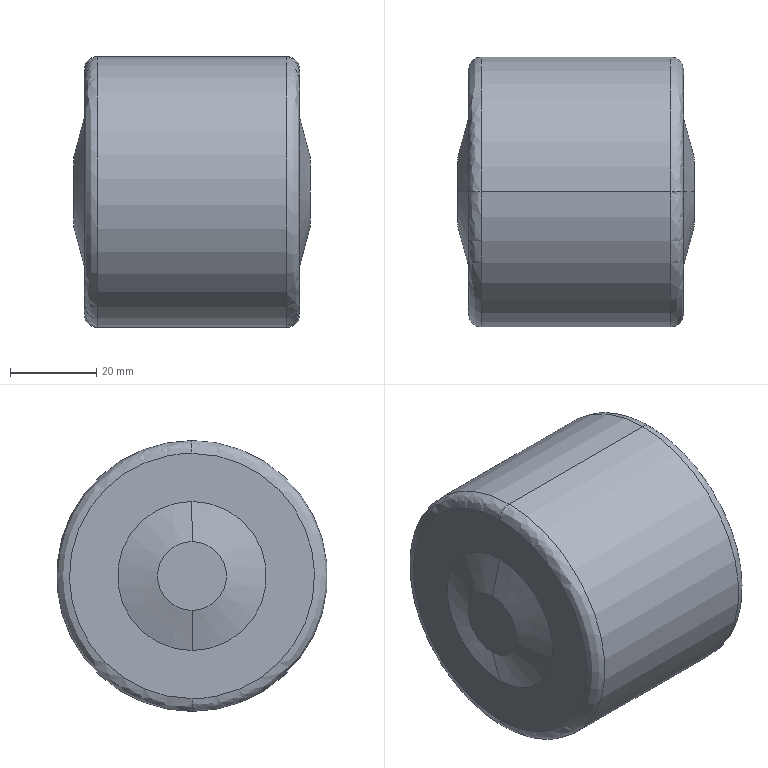Part | SolidWorks | features BaseBody 1 | 1 solid | 14 faces | box 55 x 63 x 63 mm | volume 157755 mm3 | spline 4 | cone 4 | plane 4 | cylinder 2 | commonest cylinder face diameters 63 x2
STEP:
#1=CARTESIAN_POINT('',(-22.,0.,31.5));
#2=VERTEX_POINT('',#1);
#3=CARTESIAN_POINT('',(-22.,0.,-31.5));
#4=VERTEX_POINT('',#3);
#5=CARTESIAN_POINT('',(-22.,0.,0.));
#6=DIRECTION('',(1.,0.,0.));
#7=DIRECTION('',(0.,0.,1.));
#8=AXIS2_PLACEMENT_3D('',#5,#6,#7);
#9=CIRCLE('',#8,31.5);
#10=EDGE_CURVE('',#2,#4,#9,.T.);
#11=ORIENTED_EDGE('',*,*,#10,.F.);
#12=CARTESIAN_POINT('',(-25.,0.,28.5));
#13=VERTEX_POINT('',#12);
#14=CARTESIAN_POINT('',(-22.,0.,28.5));
#15=DIRECTION('',(0.,-1.,0.));
#16=DIRECTION('',(0.,0.,1.));
#17=AXIS2_PLACEMENT_3D('',#14,#15,#16);
#18=CIRCLE('',#17,3.);
#19=EDGE_CURVE('',#2,#13,#18,.T.);
#20=ORIENTED_EDGE('',*,*,#19,.T.);
#21=CARTESIAN_POINT('',(-25.,0.,-28.5));
#22=VERTEX_POINT('',#21);
#23=CARTESIAN_POINT('',(-25.,0.,28.5));
#24=CARTESIAN_POINT('',(-25.,-57.,28.5));
#25=CARTESIAN_POINT('',(-25.,-57.,-28.5));
#26=CARTESIAN_POINT('',(-25.,0.,-28.5));
#27=(BOUNDED_CURVE()B_SPLINE_CURVE(3,(#23,#24,#25,#26),.UNSPECIFIED.,.F.,.T.)B_SPLINE_CURVE_WITH_KNOTS((4,4),(0.5,1.),.UNSPECIFIED.)CURVE()GEOMETRIC_REPRESENTATION_ITEM()RATIONAL_B_SPLINE_CURVE((1.,0.3333,0.3333,1.))REPRESENTATION_ITEM(''));
#28=EDGE_CURVE('',#13,#22,#27,.T.);
#29=ORIENTED_EDGE('',*,*,#28,.T.);
#30=CARTESIAN_POINT('',(-22.,0.,-28.5));
#31=DIRECTION('',(0.,1.,0.));
#32=DIRECTION('',(0.,0.,-1.));
#33=AXIS2_PLACEMENT_3D('',#30,#31,#32);
#34=CIRCLE('',#33,3.);
#35=EDGE_CURVE('',#4,#22,#34,.T.);
#36=ORIENTED_EDGE('',*,*,#35,.F.);
#37=EDGE_LOOP('',(#11,#20,#29,#36));
#38=FACE_OUTER_BOUND('',#37,.T.);
#39=CARTESIAN_POINT('',(-22.,0.,31.5));
#40=CARTESIAN_POINT('',(-22.,-63.,31.5));
#41=CARTESIAN_POINT('',(-22.,-63.,-31.5));
#42=CARTESIAN_POINT('',(-22.,0.,-31.5));
#43=CARTESIAN_POINT('',(-23.757,0.,31.5));
#44=CARTESIAN_POINT('',(-23.757,-63.,31.5));
#45=CARTESIAN_POINT('',(-23.757,-63.,-31.5));
#46=CARTESIAN_POINT('',(-23.757,0.,-31.5));
#47=CARTESIAN_POINT('',(-25.,0.,30.257));
#48=CARTESIAN_POINT('',(-25.,-60.515,30.257));
#49=CARTESIAN_POINT('',(-25.,-60.515,-30.257));
#50=CARTESIAN_POINT('',(-25.,0.,-30.257));
#51=CARTESIAN_POINT('',(-25.,0.,28.5));
#52=CARTESIAN_POINT('',(-25.,-57.,28.5));
#53=CARTESIAN_POINT('',(-25.,-57.,-28.5));
#54=CARTESIAN_POINT('',(-25.,0.,-28.5));
#55=(BOUNDED_SURFACE()B_SPLINE_SURFACE(3,3,((#39,#40,#41,#42),(#43,#44,#45,#46),(#47,#48,#49,#50),(#51,#52,#53,#54)),.UNSPECIFIED.,.F.,.F.,.F.)B_SPLINE_SURFACE_WITH_KNOTS((4,4),(4,4),(0.,1.),(0.,1.),.UNSPECIFIED.)GEOMETRIC_REPRESENTATION_ITEM()RATIONAL_B_SPLINE_SURFACE(((1.,0.3333,0.3333,1.),(0.8047,0.2682,0.2682,0.8047),(0.8047,0.2682,0.2682,0.8047),(1.,0.3333,0.3333,1.)))REPRESENTATION_ITEM('')SURFACE());
#56=ADVANCED_FACE('',(#38),#55,.T.);
#57=CARTESIAN_POINT('',(25.,0.,-28.5));
#58=VERTEX_POINT('',#57);
#59=CARTESIAN_POINT('',(25.,0.,28.5));
#60=VERTEX_POINT('',#59);
#61=CARTESIAN_POINT('',(25.,0.,-28.5));
#62=CARTESIAN_POINT('',(25.,-57.,-28.5));
#63=CARTESIAN_POINT('',(25.,-57.,28.5));
#64=CARTESIAN_POINT('',(25.,0.,28.5));
#65=(BOUNDED_CURVE()B_SPLINE_CURVE(3,(#61,#62,#63,#64),.UNSPECIFIED.,.F.,.F.)B_SPLINE_CURVE_WITH_KNOTS((4,4),(0.,0.5),.UNSPECIFIED.)CURVE()GEOMETRIC_REPRESENTATION_ITEM()RATIONAL_B_SPLINE_CURVE((1.,0.3333,0.3333,1.))REPRESENTATION_ITEM(''));
#66=EDGE_CURVE('',#58,#60,#65,.T.);
#67=ORIENTED_EDGE('',*,*,#66,.T.);
#68=CARTESIAN_POINT('',(22.,0.,31.5));
#69=VERTEX_POINT('',#68);
#70=CARTESIAN_POINT('',(22.,0.,28.5));
#71=DIRECTION('',(0.,-1.,0.));
#72=DIRECTION('',(0.,0.,1.));
#73=AXIS2_PLACEMENT_3D('',#70,#71,#72);
#74=CIRCLE('',#73,3.);
#75=EDGE_CURVE('',#60,#69,#74,.T.);
#76=ORIENTED_EDGE('',*,*,#75,.T.);
#77=CARTESIAN_POINT('',(22.,0.,-31.5));
#78=VERTEX_POINT('',#77);
#79=CARTESIAN_POINT('',(22.,0.,0.));
#80=DIRECTION('',(-1.,0.,0.));
#81=DIRECTION('',(0.,0.,1.));
#82=AXIS2_PLACEMENT_3D('',#79,#80,#81);
#83=CIRCLE('',#82,31.5);
#84=EDGE_CURVE('',#78,#69,#83,.T.);
#85=ORIENTED_EDGE('',*,*,#84,.F.);
#86=CARTESIAN_POINT('',(22.,0.,-28.5));
#87=DIRECTION('',(0.,1.,0.));
#88=DIRECTION('',(0.,0.,-1.));
#89=AXIS2_PLACEMENT_3D('',#86,#87,#88);
#90=CIRCLE('',#89,3.);
#91=EDGE_CURVE('',#58,#78,#90,.T.);
#92=ORIENTED_EDGE('',*,*,#91,.F.);
#93=EDGE_LOOP('',(#67,#76,#85,#92));
#94=FACE_OUTER_BOUND('',#93,.T.);
#95=CARTESIAN_POINT('',(25.,0.,28.5));
#96=CARTESIAN_POINT('',(25.,-57.,28.5));
#97=CARTESIAN_POINT('',(25.,-57.,-28.5));
#98=CARTESIAN_POINT('',(25.,0.,-28.5));
#99=CARTESIAN_POINT('',(25.,0.,30.257));
#100=CARTESIAN_POINT('',(25.,-60.515,30.257));
#101=CARTESIAN_POINT('',(25.,-60.515,-30.257));
#102=CARTESIAN_POINT('',(25.,0.,-30.257));
#103=CARTESIAN_POINT('',(23.757,0.,31.5));
#104=CARTESIAN_POINT('',(23.757,-63.,31.5));
#105=CARTESIAN_POINT('',(23.757,-63.,-31.5));
#106=CARTESIAN_POINT('',(23.757,0.,-31.5));
#107=CARTESIAN_POINT('',(22.,0.,31.5));
#108=CARTESIAN_POINT('',(22.,-63.,31.5));
#109=CARTESIAN_POINT('',(22.,-63.,-31.5));
#110=CARTESIAN_POINT('',(22.,0.,-31.5));
#111=(BOUNDED_SURFACE()B_SPLINE_SURFACE(3,3,((#95,#96,#97,#98),(#99,#100,#101,#102),(#103,#104,#105,#106),(#107,#108,#109,#110)),.UNSPECIFIED.,.F.,.F.,.T.)B_SPLINE_SURFACE_WITH_KNOTS((4,4),(4,4),(0.,1.),(0.,1.),.UNSPECIFIED.)GEOMETRIC_REPRESENTATION_ITEM()RATIONAL_B_SPLINE_SURFACE(((1.,0.3333,0.3333,1.),(0.8047,0.2682,0.2682,0.8047),(0.8047,0.2682,0.2682,0.8047),(1.,0.3333,0.3333,1.)))REPRESENTATION_ITEM('')SURFACE());
#112=ADVANCED_FACE('',(#94),#111,.T.);
#113=CARTESIAN_POINT('',(22.,0.,0.));
#114=DIRECTION('',(-1.,0.,0.));
#115=DIRECTION('',(0.,0.,1.));
#116=AXIS2_PLACEMENT_3D('',#113,#114,#115);
#117=CIRCLE('',#116,31.5);
#118=EDGE_CURVE('',#69,#78,#117,.T.);
#119=ORIENTED_EDGE('',*,*,#118,.T.);
#120=CARTESIAN_POINT('',(50.,0.,-31.5));
#121=DIRECTION('',(-1.,0.,0.));
#122=VECTOR('',#121,1000.);
#123=LINE('',#120,#122);
#124=EDGE_CURVE('',#78,#4,#123,.T.);
#125=ORIENTED_EDGE('',*,*,#124,.T.);
#126=CARTESIAN_POINT('',(-22.,0.,0.));
#127=DIRECTION('',(1.,0.,0.));
#128=DIRECTION('',(0.,0.,1.));
#129=AXIS2_PLACEMENT_3D('',#126,#127,#128);
#130=CIRCLE('',#129,31.5);
#131=EDGE_CURVE('',#4,#2,#130,.T.);
#132=ORIENTED_EDGE('',*,*,#131,.T.);
#133=CARTESIAN_POINT('',(50.,0.,31.5));
#134=DIRECTION('',(-1.,0.,0.));
#135=VECTOR('',#134,1000.);
#136=LINE('',#133,#135);
#137=EDGE_CURVE('',#69,#2,#136,.T.);
#138=ORIENTED_EDGE('',*,*,#137,.F.);
#139=EDGE_LOOP('',(#119,#125,#132,#138));
#140=FACE_OUTER_BOUND('',#139,.T.);
#141=CARTESIAN_POINT('',(50.,0.,0.));
#142=DIRECTION('',(-1.,0.,0.));
#143=DIRECTION('',(0.,0.,1.));
#144=AXIS2_PLACEMENT_3D('',#141,#142,#143);
#145=CYLINDRICAL_SURFACE('',#144,31.5);
#146=ADVANCED_FACE('',(#140),#145,.T.);
#147=CARTESIAN_POINT('',(-27.5,0.,-8.));
#148=VERTEX_POINT('',#147);
#149=CARTESIAN_POINT('',(-27.5,0.,8.));
#150=VERTEX_POINT('',#149);
#151=CARTESIAN_POINT('',(-27.5,0.,0.));
#152=DIRECTION('',(1.,0.,0.));
#153=DIRECTION('',(0.,0.,-1.));
#154=AXIS2_PLACEMENT_3D('',#151,#152,#153);
#155=CIRCLE('',#154,8.);
#156=EDGE_CURVE('',#148,#150,#155,.T.);
#157=ORIENTED_EDGE('',*,*,#156,.T.);
#158=CARTESIAN_POINT('',(-25.,0.,17.33));
#159=VERTEX_POINT('',#158);
#160=CARTESIAN_POINT('',(-25.,0.,17.33));
#161=DIRECTION('',(0.2588,0.,0.9659));
#162=VECTOR('',#161,1000.);
#163=LINE('',#160,#162);
#164=EDGE_CURVE('',#150,#159,#163,.T.);
#165=ORIENTED_EDGE('',*,*,#164,.T.);
#166=CARTESIAN_POINT('',(-25.,0.,-17.33));
#167=VERTEX_POINT('',#166);
#168=CARTESIAN_POINT('',(-25.,0.,0.));
#169=DIRECTION('',(-1.,0.,0.));
#170=DIRECTION('',(0.,0.,-1.));
#171=AXIS2_PLACEMENT_3D('',#168,#169,#170);
#172=CIRCLE('',#171,17.33);
#173=EDGE_CURVE('',#159,#167,#172,.T.);
#174=ORIENTED_EDGE('',*,*,#173,.T.);
#175=CARTESIAN_POINT('',(-25.,0.,-17.33));
#176=DIRECTION('',(0.2588,0.,-0.9659));
#177=VECTOR('',#176,1000.);
#178=LINE('',#175,#177);
#179=EDGE_CURVE('',#148,#167,#178,.T.);
#180=ORIENTED_EDGE('',*,*,#179,.F.);
#181=EDGE_LOOP('',(#157,#165,#174,#180));
#182=FACE_OUTER_BOUND('',#181,.T.);
#183=CARTESIAN_POINT('',(-25.,0.,0.));
#184=DIRECTION('',(1.,0.,0.));
#185=DIRECTION('',(0.,0.,-1.));
#186=AXIS2_PLACEMENT_3D('',#183,#184,#185);
#187=CONICAL_SURFACE('',#186,17.33,1.309);
#188=ADVANCED_FACE('',(#182),#187,.T.);
#189=CARTESIAN_POINT('',(27.5,0.,8.));
#190=VERTEX_POINT('',#189);
#191=CARTESIAN_POINT('',(27.5,0.,-8.));
#192=VERTEX_POINT('',#191);
#193=CARTESIAN_POINT('',(27.5,0.,0.));
#194=DIRECTION('',(-1.,0.,0.));
#195=DIRECTION('',(0.,0.,1.));
#196=AXIS2_PLACEMENT_3D('',#193,#194,#195);
#197=CIRCLE('',#196,8.);
#198=EDGE_CURVE('',#190,#192,#197,.T.);
#199=ORIENTED_EDGE('',*,*,#198,.T.);
#200=CARTESIAN_POINT('',(25.,0.,-17.33));
#201=VERTEX_POINT('',#200);
#202=CARTESIAN_POINT('',(25.,0.,-17.33));
#203=DIRECTION('',(-0.2588,0.,-0.9659));
#204=VECTOR('',#203,1000.);
#205=LINE('',#202,#204);
#206=EDGE_CURVE('',#192,#201,#205,.T.);
#207=ORIENTED_EDGE('',*,*,#206,.T.);
#208=CARTESIAN_POINT('',(25.,0.,17.33));
#209=VERTEX_POINT('',#208);
#210=CARTESIAN_POINT('',(25.,0.,0.));
#211=DIRECTION('',(1.,0.,0.));
#212=DIRECTION('',(0.,0.,1.));
#213=AXIS2_PLACEMENT_3D('',#210,#211,#212);
#214=CIRCLE('',#213,17.33);
#215=EDGE_CURVE('',#201,#209,#214,.T.);
#216=ORIENTED_EDGE('',*,*,#215,.T.);
#217=CARTESIAN_POINT('',(25.,0.,17.33));
#218=DIRECTION('',(-0.2588,0.,0.9659));
#219=VECTOR('',#218,1000.);
#220=LINE('',#217,#219);
#221=EDGE_CURVE('',#190,#209,#220,.T.);
#222=ORIENTED_EDGE('',*,*,#221,.F.);
#223=EDGE_LOOP('',(#199,#207,#216,#222));
#224=FACE_OUTER_BOUND('',#223,.T.);
#225=CARTESIAN_POINT('',(25.,0.,0.));
#226=DIRECTION('',(-1.,0.,0.));
#227=DIRECTION('',(0.,0.,1.));
#228=AXIS2_PLACEMENT_3D('',#225,#226,#227);
#229=CONICAL_SURFACE('',#228,17.33,1.309);
#230=ADVANCED_FACE('',(#224),#229,.T.);
#231=ORIENTED_EDGE('',*,*,#124,.F.);
#232=ORIENTED_EDGE('',*,*,#84,.T.);
#233=ORIENTED_EDGE('',*,*,#137,.T.);
#234=ORIENTED_EDGE('',*,*,#10,.T.);
#235=EDGE_LOOP('',(#231,#232,#233,#234));
#236=FACE_OUTER_BOUND('',#235,.T.);
#237=CARTESIAN_POINT('',(50.,0.,0.));
#238=DIRECTION('',(-1.,0.,0.));
#239=DIRECTION('',(0.,0.,1.));
#240=AXIS2_PLACEMENT_3D('',#237,#238,#239);
#241=CYLINDRICAL_SURFACE('',#240,31.5);
#242=ADVANCED_FACE('',(#236),#241,.T.);
#243=ORIENTED_EDGE('',*,*,#19,.F.);
#244=ORIENTED_EDGE('',*,*,#131,.F.);
#245=ORIENTED_EDGE('',*,*,#35,.T.);
#246=CARTESIAN_POINT('',(-25.,0.,-28.5));
#247=CARTESIAN_POINT('',(-25.,57.,-28.5));
#248=CARTESIAN_POINT('',(-25.,57.,28.5));
#249=CARTESIAN_POINT('',(-25.,0.,28.5));
#250=(BOUNDED_CURVE()B_SPLINE_CURVE(3,(#246,#247,#248,#249),.UNSPECIFIED.,.F.,.T.)B_SPLINE_CURVE_WITH_KNOTS((4,4),(0.,0.5),.UNSPECIFIED.)CURVE()GEOMETRIC_REPRESENTATION_ITEM()RATIONAL_B_SPLINE_CURVE((1.,0.3333,0.3333,1.))REPRESENTATION_ITEM(''));
#251=EDGE_CURVE('',#22,#13,#250,.T.);
#252=ORIENTED_EDGE('',*,*,#251,.T.);
#253=EDGE_LOOP('',(#243,#244,#245,#252));
#254=FACE_OUTER_BOUND('',#253,.T.);
#255=CARTESIAN_POINT('',(-22.,0.,-31.5));
#256=CARTESIAN_POINT('',(-22.,63.,-31.5));
#257=CARTESIAN_POINT('',(-22.,63.,31.5));
#258=CARTESIAN_POINT('',(-22.,0.,31.5));
#259=CARTESIAN_POINT('',(-23.757,0.,-31.5));
#260=CARTESIAN_POINT('',(-23.757,63.,-31.5));
#261=CARTESIAN_POINT('',(-23.757,63.,31.5));
#262=CARTESIAN_POINT('',(-23.757,0.,31.5));
#263=CARTESIAN_POINT('',(-25.,0.,-30.257));
#264=CARTESIAN_POINT('',(-25.,60.515,-30.257));
#265=CARTESIAN_POINT('',(-25.,60.515,30.257));
#266=CARTESIAN_POINT('',(-25.,0.,30.257));
#267=CARTESIAN_POINT('',(-25.,0.,-28.5));
#268=CARTESIAN_POINT('',(-25.,57.,-28.5));
#269=CARTESIAN_POINT('',(-25.,57.,28.5));
#270=CARTESIAN_POINT('',(-25.,0.,28.5));
#271=(BOUNDED_SURFACE()B_SPLINE_SURFACE(3,3,((#255,#256,#257,#258),(#259,#260,#261,#262),(#263,#264,#265,#266),(#267,#268,#269,#270)),.UNSPECIFIED.,.F.,.F.,.F.)B_SPLINE_SURFACE_WITH_KNOTS((4,4),(4,4),(0.,1.),(0.,1.),.UNSPECIFIED.)GEOMETRIC_REPRESENTATION_ITEM()RATIONAL_B_SPLINE_SURFACE(((1.,0.3333,0.3333,1.),(0.8047,0.2682,0.2682,0.8047),(0.8047,0.2682,0.2682,0.8047),(1.,0.3333,0.3333,1.)))REPRESENTATION_ITEM('')SURFACE());
#272=ADVANCED_FACE('',(#254),#271,.T.);
#273=ORIENTED_EDGE('',*,*,#75,.F.);
#274=CARTESIAN_POINT('',(25.,0.,28.5));
#275=CARTESIAN_POINT('',(25.,57.,28.5));
#276=CARTESIAN_POINT('',(25.,57.,-28.5));
#277=CARTESIAN_POINT('',(25.,0.,-28.5));
#278=(BOUNDED_CURVE()B_SPLINE_CURVE(3,(#274,#275,#276,#277),.UNSPECIFIED.,.F.,.T.)B_SPLINE_CURVE_WITH_KNOTS((4,4),(0.5,1.),.UNSPECIFIED.)CURVE()GEOMETRIC_REPRESENTATION_ITEM()RATIONAL_B_SPLINE_CURVE((1.,0.3333,0.3333,1.))REPRESENTATION_ITEM(''));
#279=EDGE_CURVE('',#60,#58,#278,.T.);
#280=ORIENTED_EDGE('',*,*,#279,.T.);
#281=ORIENTED_EDGE('',*,*,#91,.T.);
#282=ORIENTED_EDGE('',*,*,#118,.F.);
#283=EDGE_LOOP('',(#273,#280,#281,#282));
#284=FACE_OUTER_BOUND('',#283,.T.);
#285=CARTESIAN_POINT('',(25.,0.,-28.5));
#286=CARTESIAN_POINT('',(25.,57.,-28.5));
#287=CARTESIAN_POINT('',(25.,57.,28.5));
#288=CARTESIAN_POINT('',(25.,0.,28.5));
#289=CARTESIAN_POINT('',(25.,0.,-30.257));
#290=CARTESIAN_POINT('',(25.,60.515,-30.257));
#291=CARTESIAN_POINT('',(25.,60.515,30.257));
#292=CARTESIAN_POINT('',(25.,0.,30.257));
#293=CARTESIAN_POINT('',(23.757,0.,-31.5));
#294=CARTESIAN_POINT('',(23.757,63.,-31.5));
#295=CARTESIAN_POINT('',(23.757,63.,31.5));
#296=CARTESIAN_POINT('',(23.757,0.,31.5));
#297=CARTESIAN_POINT('',(22.,0.,-31.5));
#298=CARTESIAN_POINT('',(22.,63.,-31.5));
#299=CARTESIAN_POINT('',(22.,63.,31.5));
#300=CARTESIAN_POINT('',(22.,0.,31.5));
#301=(BOUNDED_SURFACE()B_SPLINE_SURFACE(3,3,((#285,#286,#287,#288),(#289,#290,#291,#292),(#293,#294,#295,#296),(#297,#298,#299,#300)),.UNSPECIFIED.,.F.,.F.,.T.)B_SPLINE_SURFACE_WITH_KNOTS((4,4),(4,4),(0.,1.),(0.,1.),.UNSPECIFIED.)GEOMETRIC_REPRESENTATION_ITEM()RATIONAL_B_SPLINE_SURFACE(((1.,0.3333,0.3333,1.),(0.8047,0.2682,0.2682,0.8047),(0.8047,0.2682,0.2682,0.8047),(1.,0.3333,0.3333,1.)))REPRESENTATION_ITEM('')SURFACE());
#302=ADVANCED_FACE('',(#284),#301,.T.);
#303=CARTESIAN_POINT('',(-25.,0.,0.));
#304=DIRECTION('',(-1.,0.,0.));
#305=DIRECTION('',(0.,0.,-1.));
#306=AXIS2_PLACEMENT_3D('',#303,#304,#305);
#307=CIRCLE('',#306,17.33);
#308=EDGE_CURVE('',#167,#159,#307,.T.);
#309=ORIENTED_EDGE('',*,*,#308,.F.);
#310=ORIENTED_EDGE('',*,*,#173,.F.);
#311=EDGE_LOOP('',(#309,#310));
#312=FACE_BOUND('',#311,.T.);
#313=ORIENTED_EDGE('',*,*,#251,.F.);
#314=ORIENTED_EDGE('',*,*,#28,.F.);
#315=EDGE_LOOP('',(#313,#314));
#316=FACE_OUTER_BOUND('',#315,.T.);
#317=CARTESIAN_POINT('',(-25.,17.33,0.));
#318=DIRECTION('',(1.,0.,0.));
#319=DIRECTION('',(0.,0.,-1.));
#320=AXIS2_PLACEMENT_3D('',#317,#318,#319);
#321=PLANE('',#320);
#322=ADVANCED_FACE('',(#312,#316),#321,.F.);
#323=ORIENTED_EDGE('',*,*,#66,.F.);
#324=ORIENTED_EDGE('',*,*,#279,.F.);
#325=EDGE_LOOP('',(#323,#324));
#326=FACE_OUTER_BOUND('',#325,.T.);
#327=CARTESIAN_POINT('',(25.,0.,0.));
#328=DIRECTION('',(1.,0.,0.));
#329=DIRECTION('',(0.,0.,1.));
#330=AXIS2_PLACEMENT_3D('',#327,#328,#329);
#331=CIRCLE('',#330,17.33);
#332=EDGE_CURVE('',#209,#201,#331,.T.);
#333=ORIENTED_EDGE('',*,*,#332,.F.);
#334=ORIENTED_EDGE('',*,*,#215,.F.);
#335=EDGE_LOOP('',(#333,#334));
#336=FACE_BOUND('',#335,.T.);
#337=CARTESIAN_POINT('',(25.,28.5,0.));
#338=DIRECTION('',(-1.,0.,0.));
#339=DIRECTION('',(0.,0.,1.));
#340=AXIS2_PLACEMENT_3D('',#337,#338,#339);
#341=PLANE('',#340);
#342=ADVANCED_FACE('',(#326,#336),#341,.F.);
#343=ORIENTED_EDGE('',*,*,#164,.F.);
#344=CARTESIAN_POINT('',(-27.5,0.,0.));
#345=DIRECTION('',(1.,0.,0.));
#346=DIRECTION('',(0.,0.,-1.));
#347=AXIS2_PLACEMENT_3D('',#344,#345,#346);
#348=CIRCLE('',#347,8.);
#349=EDGE_CURVE('',#150,#148,#348,.T.);
#350=ORIENTED_EDGE('',*,*,#349,.T.);
#351=ORIENTED_EDGE('',*,*,#179,.T.);
#352=ORIENTED_EDGE('',*,*,#308,.T.);
#353=EDGE_LOOP('',(#343,#350,#351,#352));
#354=FACE_OUTER_BOUND('',#353,.T.);
#355=CARTESIAN_POINT('',(-25.,0.,0.));
#356=DIRECTION('',(1.,0.,0.));
#357=DIRECTION('',(0.,0.,-1.));
#358=AXIS2_PLACEMENT_3D('',#355,#356,#357);
#359=CONICAL_SURFACE('',#358,17.33,1.309);
#360=ADVANCED_FACE('',(#354),#359,.T.);
#361=ORIENTED_EDGE('',*,*,#206,.F.);
#362=CARTESIAN_POINT('',(27.5,0.,0.));
#363=DIRECTION('',(-1.,0.,0.));
#364=DIRECTION('',(0.,0.,1.));
#365=AXIS2_PLACEMENT_3D('',#362,#363,#364);
#366=CIRCLE('',#365,8.);
#367=EDGE_CURVE('',#192,#190,#366,.T.);
#368=ORIENTED_EDGE('',*,*,#367,.T.);
#369=ORIENTED_EDGE('',*,*,#221,.T.);
#370=ORIENTED_EDGE('',*,*,#332,.T.);
#371=EDGE_LOOP('',(#361,#368,#369,#370));
#372=FACE_OUTER_BOUND('',#371,.T.);
#373=CARTESIAN_POINT('',(25.,0.,0.));
#374=DIRECTION('',(-1.,0.,0.));
#375=DIRECTION('',(0.,0.,1.));
#376=AXIS2_PLACEMENT_3D('',#373,#374,#375);
#377=CONICAL_SURFACE('',#376,17.33,1.309);
#378=ADVANCED_FACE('',(#372),#377,.T.);
#379=ORIENTED_EDGE('',*,*,#156,.F.);
#380=ORIENTED_EDGE('',*,*,#349,.F.);
#381=EDGE_LOOP('',(#379,#380));
#382=FACE_OUTER_BOUND('',#381,.T.);
#383=CARTESIAN_POINT('',(-27.5,0.,0.));
#384=DIRECTION('',(1.,0.,0.));
#385=DIRECTION('',(0.,0.,-1.));
#386=AXIS2_PLACEMENT_3D('',#383,#384,#385);
#387=PLANE('',#386);
#388=ADVANCED_FACE('',(#382),#387,.F.);
#389=ORIENTED_EDGE('',*,*,#198,.F.);
#390=ORIENTED_EDGE('',*,*,#367,.F.);
#391=EDGE_LOOP('',(#389,#390));
#392=FACE_OUTER_BOUND('',#391,.T.);
#393=CARTESIAN_POINT('',(27.5,8.,0.));
#394=DIRECTION('',(-1.,0.,0.));
#395=DIRECTION('',(0.,0.,1.));
#396=AXIS2_PLACEMENT_3D('',#393,#394,#395);
#397=PLANE('',#396);
#398=ADVANCED_FACE('',(#392),#397,.F.);
#399=CLOSED_SHELL('',(#56,#112,#146,#188,#230,#242,#272,#302,#322,#342,#360,#378,#388,#398));
#400=MANIFOLD_SOLID_BREP('',#399);
#401=CARTESIAN_POINT('',(0.,0.,0.));
#402=DIRECTION('',(0.,0.,1.));
#403=DIRECTION('',(1.,0.,0.));
#404=AXIS2_PLACEMENT_3D('',#401,#402,#403);
#405=(LENGTH_UNIT()NAMED_UNIT(*)SI_UNIT(.MILLI.,.METRE.));
#406=UNCERTAINTY_MEASURE_WITH_UNIT(LENGTH_MEASURE(0.00001),#405,'','');
#407=(NAMED_UNIT(*)PLANE_ANGLE_UNIT()SI_UNIT($,.RADIAN.));
#408=(NAMED_UNIT(*)SI_UNIT($,.STERADIAN.)SOLID_ANGLE_UNIT());
#409=(GEOMETRIC_REPRESENTATION_CONTEXT(3)GLOBAL_UNCERTAINTY_ASSIGNED_CONTEXT((#406))GLOBAL_UNIT_ASSIGNED_CONTEXT((#405,#407,#408))REPRESENTATION_CONTEXT('',''));
#410=ADVANCED_BREP_SHAPE_REPRESENTATION('',(#400,#404),#409);